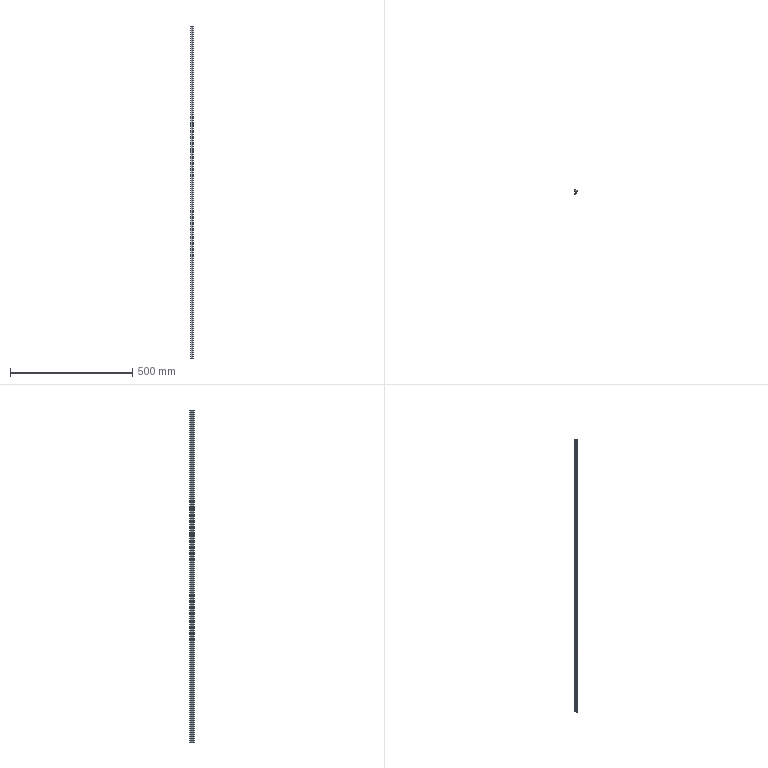Part | SolidWorks | features BaseBody 1, MoveFace 1 | 1 solid | 20 faces | box 10.8 x 17.5 x 1358 mm | volume 107011 mm3 | cylinder 11 | plane 9 | commonest cylinder face diameters 1.6 x2 14 x2 0.4 x1 0.6 x1 0.8 x1 2.6 x1
STEP:
#1=CARTESIAN_POINT('',(-3.236,-11.055,1258.));
#2=VERTEX_POINT('',#1);
#3=CARTESIAN_POINT('',(-4.3,-10.3,1258.));
#4=VERTEX_POINT('',#3);
#5=CARTESIAN_POINT('',(-3.5,-10.3,1258.));
#6=DIRECTION('',(0.,0.,-1.));
#7=DIRECTION('',(1.,0.,0.));
#8=AXIS2_PLACEMENT_3D('',#5,#6,#7);
#9=CIRCLE('',#8,0.8);
#10=EDGE_CURVE('',#2,#4,#9,.T.);
#11=ORIENTED_EDGE('',*,*,#10,.T.);
#12=CARTESIAN_POINT('',(-4.3,-10.3,-100.));
#13=VERTEX_POINT('',#12);
#14=CARTESIAN_POINT('',(-4.3,-10.3,-100.));
#15=DIRECTION('',(0.,0.,-1.));
#16=VECTOR('',#15,1000.);
#17=LINE('',#14,#16);
#18=EDGE_CURVE('',#4,#13,#17,.T.);
#19=ORIENTED_EDGE('',*,*,#18,.T.);
#20=CARTESIAN_POINT('',(-3.236,-11.055,-100.));
#21=VERTEX_POINT('',#20);
#22=CARTESIAN_POINT('',(-3.5,-10.3,-100.));
#23=DIRECTION('',(0.,0.,1.));
#24=DIRECTION('',(-1.,0.,0.));
#25=AXIS2_PLACEMENT_3D('',#22,#23,#24);
#26=CIRCLE('',#25,0.8);
#27=EDGE_CURVE('',#13,#21,#26,.T.);
#28=ORIENTED_EDGE('',*,*,#27,.T.);
#29=CARTESIAN_POINT('',(-3.236,-11.055,-100.));
#30=DIRECTION('',(0.,0.,-1.));
#31=VECTOR('',#30,1000.);
#32=LINE('',#29,#31);
#33=EDGE_CURVE('',#2,#21,#32,.T.);
#34=ORIENTED_EDGE('',*,*,#33,.F.);
#35=EDGE_LOOP('',(#11,#19,#28,#34));
#36=FACE_OUTER_BOUND('',#35,.T.);
#37=CARTESIAN_POINT('',(-3.5,-10.3,-100.));
#38=DIRECTION('',(0.,0.,-1.));
#39=DIRECTION('',(-1.,0.,0.));
#40=AXIS2_PLACEMENT_3D('',#37,#38,#39);
#41=CYLINDRICAL_SURFACE('',#40,0.8);
#42=ADVANCED_FACE('',(#36),#41,.T.);
#43=CARTESIAN_POINT('',(1.184,-6.397,-100.));
#44=VERTEX_POINT('',#43);
#45=CARTESIAN_POINT('',(-5.702,-4.29,-100.));
#46=DIRECTION('',(0.,0.,1.));
#47=DIRECTION('',(-1.,0.,0.));
#48=AXIS2_PLACEMENT_3D('',#45,#46,#47);
#49=CIRCLE('',#48,7.201);
#50=EDGE_CURVE('',#21,#44,#49,.T.);
#51=ORIENTED_EDGE('',*,*,#50,.T.);
#52=CARTESIAN_POINT('',(1.184,-6.397,1258.));
#53=VERTEX_POINT('',#52);
#54=CARTESIAN_POINT('',(1.184,-6.397,-100.));
#55=DIRECTION('',(0.,0.,1.));
#56=VECTOR('',#55,1000.);
#57=LINE('',#54,#56);
#58=EDGE_CURVE('',#44,#53,#57,.T.);
#59=ORIENTED_EDGE('',*,*,#58,.T.);
#60=CARTESIAN_POINT('',(-5.702,-4.29,1258.));
#61=DIRECTION('',(0.,0.,-1.));
#62=DIRECTION('',(1.,0.,0.));
#63=AXIS2_PLACEMENT_3D('',#60,#61,#62);
#64=CIRCLE('',#63,7.201);
#65=EDGE_CURVE('',#53,#2,#64,.T.);
#66=ORIENTED_EDGE('',*,*,#65,.T.);
#67=ORIENTED_EDGE('',*,*,#33,.T.);
#68=EDGE_LOOP('',(#51,#59,#66,#67));
#69=FACE_OUTER_BOUND('',#68,.T.);
#70=CARTESIAN_POINT('',(-5.702,-4.29,-100.));
#71=DIRECTION('',(0.,0.,-1.));
#72=DIRECTION('',(-1.,0.,0.));
#73=AXIS2_PLACEMENT_3D('',#70,#71,#72);
#74=CYLINDRICAL_SURFACE('',#73,7.201);
#75=ADVANCED_FACE('',(#69),#74,.T.);
#76=CARTESIAN_POINT('',(0.9,-6.,-100.));
#77=VERTEX_POINT('',#76);
#78=CARTESIAN_POINT('',(0.9,-6.3,-100.));
#79=DIRECTION('',(0.,0.,1.));
#80=DIRECTION('',(-1.,0.,0.));
#81=AXIS2_PLACEMENT_3D('',#78,#79,#80);
#82=CIRCLE('',#81,0.3);
#83=EDGE_CURVE('',#44,#77,#82,.T.);
#84=ORIENTED_EDGE('',*,*,#83,.T.);
#85=CARTESIAN_POINT('',(0.9,-6.,1258.));
#86=VERTEX_POINT('',#85);
#87=CARTESIAN_POINT('',(0.9,-6.,-100.));
#88=DIRECTION('',(0.,0.,1.));
#89=VECTOR('',#88,1000.);
#90=LINE('',#87,#89);
#91=EDGE_CURVE('',#77,#86,#90,.T.);
#92=ORIENTED_EDGE('',*,*,#91,.T.);
#93=CARTESIAN_POINT('',(0.9,-6.3,1258.));
#94=DIRECTION('',(0.,0.,-1.));
#95=DIRECTION('',(1.,0.,0.));
#96=AXIS2_PLACEMENT_3D('',#93,#94,#95);
#97=CIRCLE('',#96,0.3);
#98=EDGE_CURVE('',#86,#53,#97,.T.);
#99=ORIENTED_EDGE('',*,*,#98,.T.);
#100=ORIENTED_EDGE('',*,*,#58,.F.);
#101=EDGE_LOOP('',(#84,#92,#99,#100));
#102=FACE_OUTER_BOUND('',#101,.T.);
#103=CARTESIAN_POINT('',(0.9,-6.3,-100.));
#104=DIRECTION('',(0.,0.,-1.));
#105=DIRECTION('',(-1.,0.,0.));
#106=AXIS2_PLACEMENT_3D('',#103,#104,#105);
#107=CYLINDRICAL_SURFACE('',#106,0.3);
#108=ADVANCED_FACE('',(#102),#107,.T.);
#109=CARTESIAN_POINT('',(-2.5,-0.5,-100.));
#110=VERTEX_POINT('',#109);
#111=CARTESIAN_POINT('',(-2.5,-6.153,-100.));
#112=VERTEX_POINT('',#111);
#113=CARTESIAN_POINT('',(-2.5,-6.397,-100.));
#114=DIRECTION('',(0.,-1.,0.));
#115=VECTOR('',#114,1000.);
#116=LINE('',#113,#115);
#117=EDGE_CURVE('',#110,#112,#116,.T.);
#118=ORIENTED_EDGE('',*,*,#117,.F.);
#119=CARTESIAN_POINT('',(-4.2,1.695,-100.));
#120=VERTEX_POINT('',#119);
#121=CARTESIAN_POINT('',(-1.701,1.875,-100.));
#122=DIRECTION('',(0.,0.,1.));
#123=DIRECTION('',(-1.,0.,0.));
#124=AXIS2_PLACEMENT_3D('',#121,#122,#123);
#125=CIRCLE('',#124,2.506);
#126=EDGE_CURVE('',#120,#110,#125,.T.);
#127=ORIENTED_EDGE('',*,*,#126,.F.);
#128=CARTESIAN_POINT('',(-4.2,5.1,-100.));
#129=VERTEX_POINT('',#128);
#130=CARTESIAN_POINT('',(-4.2,-6.397,-100.));
#131=DIRECTION('',(0.,-1.,0.));
#132=VECTOR('',#131,1000.);
#133=LINE('',#130,#132);
#134=EDGE_CURVE('',#129,#120,#133,.T.);
#135=ORIENTED_EDGE('',*,*,#134,.F.);
#136=CARTESIAN_POINT('',(-2.892,6.4,-100.));
#137=VERTEX_POINT('',#136);
#138=CARTESIAN_POINT('',(-2.9,5.1,-100.));
#139=DIRECTION('',(0.,0.,1.));
#140=DIRECTION('',(-1.,0.,0.));
#141=AXIS2_PLACEMENT_3D('',#138,#139,#140);
#142=CIRCLE('',#141,1.3);
#143=EDGE_CURVE('',#137,#129,#142,.T.);
#144=ORIENTED_EDGE('',*,*,#143,.F.);
#145=CARTESIAN_POINT('',(0.5,5.5,-100.));
#146=VERTEX_POINT('',#145);
#147=CARTESIAN_POINT('',(-2.934,-0.5999,-100.));
#148=DIRECTION('',(0.,0.,1.));
#149=DIRECTION('',(-1.,0.,0.));
#150=AXIS2_PLACEMENT_3D('',#147,#148,#149);
#151=CIRCLE('',#150,7.);
#152=EDGE_CURVE('',#146,#137,#151,.T.);
#153=ORIENTED_EDGE('',*,*,#152,.F.);
#154=CARTESIAN_POINT('',(5.5,1.7,-100.));
#155=VERTEX_POINT('',#154);
#156=CARTESIAN_POINT('',(5.5,1.7,-100.));
#157=DIRECTION('',(-0.7962,0.6051,0.));
#158=VECTOR('',#157,1000.);
#159=LINE('',#156,#158);
#160=EDGE_CURVE('',#155,#146,#159,.T.);
#161=ORIENTED_EDGE('',*,*,#160,.F.);
#162=CARTESIAN_POINT('',(6.458,-0.2215,-100.));
#163=VERTEX_POINT('',#162);
#164=CARTESIAN_POINT('',(6.458,-0.2215,-100.));
#165=DIRECTION('',(-0.4462,0.8949,0.));
#166=VECTOR('',#165,1000.);
#167=LINE('',#164,#166);
#168=EDGE_CURVE('',#163,#155,#167,.T.);
#169=ORIENTED_EDGE('',*,*,#168,.F.);
#170=CARTESIAN_POINT('',(5.895,-0.7433,-100.));
#171=VERTEX_POINT('',#170);
#172=CARTESIAN_POINT('',(6.1,-0.4,-100.));
#173=DIRECTION('',(0.,0.,1.));
#174=DIRECTION('',(-1.,0.,0.));
#175=AXIS2_PLACEMENT_3D('',#172,#173,#174);
#176=CIRCLE('',#175,0.4);
#177=EDGE_CURVE('',#171,#163,#176,.T.);
#178=ORIENTED_EDGE('',*,*,#177,.F.);
#179=CARTESIAN_POINT('',(3.,0.,-100.));
#180=VERTEX_POINT('',#179);
#181=CARTESIAN_POINT('',(2.746,-6.995,-100.));
#182=DIRECTION('',(0.,0.,-1.));
#183=DIRECTION('',(-1.,0.,0.));
#184=AXIS2_PLACEMENT_3D('',#181,#182,#183);
#185=CIRCLE('',#184,7.);
#186=EDGE_CURVE('',#180,#171,#185,.T.);
#187=ORIENTED_EDGE('',*,*,#186,.F.);
#188=CARTESIAN_POINT('',(0.,0.,-100.));
#189=VERTEX_POINT('',#188);
#190=CARTESIAN_POINT('',(-6.814,0.,-100.));
#191=DIRECTION('',(1.,0.,0.));
#192=VECTOR('',#191,1000.);
#193=LINE('',#190,#192);
#194=EDGE_CURVE('',#189,#180,#193,.T.);
#195=ORIENTED_EDGE('',*,*,#194,.F.);
#196=CARTESIAN_POINT('',(0.,-5.8,-100.));
#197=VERTEX_POINT('',#196);
#198=CARTESIAN_POINT('',(0.,-6.397,-100.));
#199=DIRECTION('',(0.,1.,0.));
#200=VECTOR('',#199,1000.);
#201=LINE('',#198,#200);
#202=EDGE_CURVE('',#197,#189,#201,.T.);
#203=ORIENTED_EDGE('',*,*,#202,.F.);
#204=CARTESIAN_POINT('',(0.2,-6.,-100.));
#205=VERTEX_POINT('',#204);
#206=CARTESIAN_POINT('',(0.2,-5.8,-100.));
#207=DIRECTION('',(0.,0.,1.));
#208=DIRECTION('',(-1.,0.,0.));
#209=AXIS2_PLACEMENT_3D('',#206,#207,#208);
#210=CIRCLE('',#209,0.2);
#211=EDGE_CURVE('',#197,#205,#210,.T.);
#212=ORIENTED_EDGE('',*,*,#211,.T.);
#213=CARTESIAN_POINT('',(-6.814,-6.,-100.));
#214=DIRECTION('',(-1.,0.,0.));
#215=VECTOR('',#214,1000.);
#216=LINE('',#213,#215);
#217=EDGE_CURVE('',#77,#205,#216,.T.);
#218=ORIENTED_EDGE('',*,*,#217,.F.);
#219=ORIENTED_EDGE('',*,*,#83,.F.);
#220=ORIENTED_EDGE('',*,*,#50,.F.);
#221=ORIENTED_EDGE('',*,*,#27,.F.);
#222=CARTESIAN_POINT('',(-3.998,-9.674,-100.));
#223=VERTEX_POINT('',#222);
#224=CARTESIAN_POINT('',(-3.5,-10.3,-100.));
#225=DIRECTION('',(0.,0.,1.));
#226=DIRECTION('',(-1.,0.,0.));
#227=AXIS2_PLACEMENT_3D('',#224,#225,#226);
#228=CIRCLE('',#227,0.8);
#229=EDGE_CURVE('',#223,#13,#228,.T.);
#230=ORIENTED_EDGE('',*,*,#229,.F.);
#231=CARTESIAN_POINT('',(-6.814,-6.397,-100.));
#232=DIRECTION('',(0.,0.,-1.));
#233=DIRECTION('',(-1.,0.,0.));
#234=AXIS2_PLACEMENT_3D('',#231,#232,#233);
#235=CIRCLE('',#234,4.321);
#236=EDGE_CURVE('',#112,#223,#235,.T.);
#237=ORIENTED_EDGE('',*,*,#236,.F.);
#238=EDGE_LOOP('',(#118,#127,#135,#144,#153,#161,#169,#178,#187,#195,#203,#212,#218,#219,#220,#221,#230,#237));
#239=FACE_OUTER_BOUND('',#238,.T.);
#240=CARTESIAN_POINT('',(-6.814,-6.397,-100.));
#241=DIRECTION('',(0.,0.,1.));
#242=DIRECTION('',(1.,0.,0.));
#243=AXIS2_PLACEMENT_3D('',#240,#241,#242);
#244=PLANE('',#243);
#245=ADVANCED_FACE('',(#239),#244,.F.);
#246=ORIENTED_EDGE('',*,*,#18,.F.);
#247=CARTESIAN_POINT('',(-3.998,-9.674,1258.));
#248=VERTEX_POINT('',#247);
#249=CARTESIAN_POINT('',(-3.5,-10.3,1258.));
#250=DIRECTION('',(0.,0.,-1.));
#251=DIRECTION('',(1.,0.,0.));
#252=AXIS2_PLACEMENT_3D('',#249,#250,#251);
#253=CIRCLE('',#252,0.8);
#254=EDGE_CURVE('',#4,#248,#253,.T.);
#255=ORIENTED_EDGE('',*,*,#254,.T.);
#256=CARTESIAN_POINT('',(-3.998,-9.674,-100.));
#257=DIRECTION('',(0.,0.,-1.));
#258=VECTOR('',#257,1000.);
#259=LINE('',#256,#258);
#260=EDGE_CURVE('',#248,#223,#259,.T.);
#261=ORIENTED_EDGE('',*,*,#260,.T.);
#262=ORIENTED_EDGE('',*,*,#229,.T.);
#263=EDGE_LOOP('',(#246,#255,#261,#262));
#264=FACE_OUTER_BOUND('',#263,.T.);
#265=CARTESIAN_POINT('',(-3.5,-10.3,-100.));
#266=DIRECTION('',(0.,0.,-1.));
#267=DIRECTION('',(-1.,0.,0.));
#268=AXIS2_PLACEMENT_3D('',#265,#266,#267);
#269=CYLINDRICAL_SURFACE('',#268,0.8);
#270=ADVANCED_FACE('',(#264),#269,.T.);
#271=CARTESIAN_POINT('',(-4.2,1.695,1258.));
#272=VERTEX_POINT('',#271);
#273=CARTESIAN_POINT('',(-2.5,-0.5,1258.));
#274=VERTEX_POINT('',#273);
#275=CARTESIAN_POINT('',(-1.701,1.875,1258.));
#276=DIRECTION('',(0.,0.,1.));
#277=DIRECTION('',(1.,0.,0.));
#278=AXIS2_PLACEMENT_3D('',#275,#276,#277);
#279=CIRCLE('',#278,2.506);
#280=EDGE_CURVE('',#272,#274,#279,.T.);
#281=ORIENTED_EDGE('',*,*,#280,.T.);
#282=CARTESIAN_POINT('',(-2.5,-6.153,1258.));
#283=VERTEX_POINT('',#282);
#284=CARTESIAN_POINT('',(-2.5,-6.397,1258.));
#285=DIRECTION('',(0.,-1.,0.));
#286=VECTOR('',#285,1000.);
#287=LINE('',#284,#286);
#288=EDGE_CURVE('',#274,#283,#287,.T.);
#289=ORIENTED_EDGE('',*,*,#288,.T.);
#290=CARTESIAN_POINT('',(-6.814,-6.397,1258.));
#291=DIRECTION('',(0.,0.,-1.));
#292=DIRECTION('',(1.,0.,0.));
#293=AXIS2_PLACEMENT_3D('',#290,#291,#292);
#294=CIRCLE('',#293,4.321);
#295=EDGE_CURVE('',#283,#248,#294,.T.);
#296=ORIENTED_EDGE('',*,*,#295,.T.);
#297=ORIENTED_EDGE('',*,*,#254,.F.);
#298=ORIENTED_EDGE('',*,*,#10,.F.);
#299=ORIENTED_EDGE('',*,*,#65,.F.);
#300=ORIENTED_EDGE('',*,*,#98,.F.);
#301=CARTESIAN_POINT('',(0.2,-6.,1258.));
#302=VERTEX_POINT('',#301);
#303=CARTESIAN_POINT('',(-6.814,-6.,1258.));
#304=DIRECTION('',(-1.,0.,0.));
#305=VECTOR('',#304,1000.);
#306=LINE('',#303,#305);
#307=EDGE_CURVE('',#86,#302,#306,.T.);
#308=ORIENTED_EDGE('',*,*,#307,.T.);
#309=CARTESIAN_POINT('',(0.,-5.8,1258.));
#310=VERTEX_POINT('',#309);
#311=CARTESIAN_POINT('',(0.2,-5.8,1258.));
#312=DIRECTION('',(0.,0.,-1.));
#313=DIRECTION('',(1.,0.,0.));
#314=AXIS2_PLACEMENT_3D('',#311,#312,#313);
#315=CIRCLE('',#314,0.2);
#316=EDGE_CURVE('',#302,#310,#315,.T.);
#317=ORIENTED_EDGE('',*,*,#316,.T.);
#318=CARTESIAN_POINT('',(0.,0.,1258.));
#319=VERTEX_POINT('',#318);
#320=CARTESIAN_POINT('',(0.,-6.397,1258.));
#321=DIRECTION('',(0.,1.,0.));
#322=VECTOR('',#321,1000.);
#323=LINE('',#320,#322);
#324=EDGE_CURVE('',#310,#319,#323,.T.);
#325=ORIENTED_EDGE('',*,*,#324,.T.);
#326=CARTESIAN_POINT('',(3.,0.,1258.));
#327=VERTEX_POINT('',#326);
#328=CARTESIAN_POINT('',(-6.814,0.,1258.));
#329=DIRECTION('',(1.,0.,0.));
#330=VECTOR('',#329,1000.);
#331=LINE('',#328,#330);
#332=EDGE_CURVE('',#319,#327,#331,.T.);
#333=ORIENTED_EDGE('',*,*,#332,.T.);
#334=CARTESIAN_POINT('',(5.895,-0.7433,1258.));
#335=VERTEX_POINT('',#334);
#336=CARTESIAN_POINT('',(2.746,-6.995,1258.));
#337=DIRECTION('',(0.,0.,-1.));
#338=DIRECTION('',(1.,0.,0.));
#339=AXIS2_PLACEMENT_3D('',#336,#337,#338);
#340=CIRCLE('',#339,7.);
#341=EDGE_CURVE('',#327,#335,#340,.T.);
#342=ORIENTED_EDGE('',*,*,#341,.T.);
#343=CARTESIAN_POINT('',(6.458,-0.2215,1258.));
#344=VERTEX_POINT('',#343);
#345=CARTESIAN_POINT('',(6.1,-0.4,1258.));
#346=DIRECTION('',(0.,0.,-1.));
#347=DIRECTION('',(1.,0.,0.));
#348=AXIS2_PLACEMENT_3D('',#345,#346,#347);
#349=CIRCLE('',#348,0.4);
#350=EDGE_CURVE('',#344,#335,#349,.T.);
#351=ORIENTED_EDGE('',*,*,#350,.F.);
#352=CARTESIAN_POINT('',(5.5,1.7,1258.));
#353=VERTEX_POINT('',#352);
#354=CARTESIAN_POINT('',(6.282,0.1323,1258.));
#355=DIRECTION('',(-0.4462,0.8949,0.));
#356=VECTOR('',#355,1000.);
#357=LINE('',#354,#356);
#358=EDGE_CURVE('',#344,#353,#357,.T.);
#359=ORIENTED_EDGE('',*,*,#358,.T.);
#360=CARTESIAN_POINT('',(0.5,5.5,1258.));
#361=VERTEX_POINT('',#360);
#362=CARTESIAN_POINT('',(1.595,4.668,1258.));
#363=DIRECTION('',(-0.7962,0.6051,0.));
#364=VECTOR('',#363,1000.);
#365=LINE('',#362,#364);
#366=EDGE_CURVE('',#353,#361,#365,.T.);
#367=ORIENTED_EDGE('',*,*,#366,.T.);
#368=CARTESIAN_POINT('',(-2.892,6.4,1258.));
#369=VERTEX_POINT('',#368);
#370=CARTESIAN_POINT('',(-2.934,-0.5999,1258.));
#371=DIRECTION('',(0.,0.,1.));
#372=DIRECTION('',(1.,0.,0.));
#373=AXIS2_PLACEMENT_3D('',#370,#371,#372);
#374=CIRCLE('',#373,7.);
#375=EDGE_CURVE('',#361,#369,#374,.T.);
#376=ORIENTED_EDGE('',*,*,#375,.T.);
#377=CARTESIAN_POINT('',(-4.2,5.1,1258.));
#378=VERTEX_POINT('',#377);
#379=CARTESIAN_POINT('',(-2.9,5.1,1258.));
#380=DIRECTION('',(0.,0.,1.));
#381=DIRECTION('',(1.,0.,0.));
#382=AXIS2_PLACEMENT_3D('',#379,#380,#381);
#383=CIRCLE('',#382,1.3);
#384=EDGE_CURVE('',#369,#378,#383,.T.);
#385=ORIENTED_EDGE('',*,*,#384,.T.);
#386=CARTESIAN_POINT('',(-4.2,-6.397,1258.));
#387=DIRECTION('',(0.,-1.,0.));
#388=VECTOR('',#387,1000.);
#389=LINE('',#386,#388);
#390=EDGE_CURVE('',#378,#272,#389,.T.);
#391=ORIENTED_EDGE('',*,*,#390,.T.);
#392=EDGE_LOOP('',(#281,#289,#296,#297,#298,#299,#300,#308,#317,#325,#333,#342,#351,#359,#367,#376,#385,#391));
#393=FACE_OUTER_BOUND('',#392,.T.);
#394=CARTESIAN_POINT('',(-6.814,-6.397,1258.));
#395=DIRECTION('',(0.,0.,1.));
#396=DIRECTION('',(1.,0.,0.));
#397=AXIS2_PLACEMENT_3D('',#394,#395,#396);
#398=PLANE('',#397);
#399=ADVANCED_FACE('',(#393),#398,.T.);
#400=ORIENTED_EDGE('',*,*,#217,.T.);
#401=CARTESIAN_POINT('',(0.2,-6.,-100.));
#402=DIRECTION('',(0.,0.,1.));
#403=VECTOR('',#402,1000.);
#404=LINE('',#401,#403);
#405=EDGE_CURVE('',#205,#302,#404,.T.);
#406=ORIENTED_EDGE('',*,*,#405,.T.);
#407=ORIENTED_EDGE('',*,*,#307,.F.);
#408=ORIENTED_EDGE('',*,*,#91,.F.);
#409=EDGE_LOOP('',(#400,#406,#407,#408));
#410=FACE_OUTER_BOUND('',#409,.T.);
#411=CARTESIAN_POINT('',(0.9,-6.,-100.));
#412=DIRECTION('',(0.,1.,0.));
#413=DIRECTION('',(0.,0.,1.));
#414=AXIS2_PLACEMENT_3D('',#411,#412,#413);
#415=PLANE('',#414);
#416=ADVANCED_FACE('',(#410),#415,.T.);
#417=CARTESIAN_POINT('',(-2.5,-6.153,-100.));
#418=DIRECTION('',(0.,0.,1.));
#419=VECTOR('',#418,1000.);
#420=LINE('',#417,#419);
#421=EDGE_CURVE('',#112,#283,#420,.T.);
#422=ORIENTED_EDGE('',*,*,#421,.F.);
#423=ORIENTED_EDGE('',*,*,#236,.T.);
#424=ORIENTED_EDGE('',*,*,#260,.F.);
#425=ORIENTED_EDGE('',*,*,#295,.F.);
#426=EDGE_LOOP('',(#422,#423,#424,#425));
#427=FACE_OUTER_BOUND('',#426,.T.);
#428=CARTESIAN_POINT('',(-6.814,-6.397,-100.));
#429=DIRECTION('',(0.,0.,-1.));
#430=DIRECTION('',(-1.,0.,0.));
#431=AXIS2_PLACEMENT_3D('',#428,#429,#430);
#432=CYLINDRICAL_SURFACE('',#431,4.321);
#433=ADVANCED_FACE('',(#427),#432,.F.);
#434=ORIENTED_EDGE('',*,*,#117,.T.);
#435=ORIENTED_EDGE('',*,*,#421,.T.);
#436=ORIENTED_EDGE('',*,*,#288,.F.);
#437=CARTESIAN_POINT('',(-2.5,-0.5,-100.));
#438=DIRECTION('',(0.,0.,-1.));
#439=VECTOR('',#438,1000.);
#440=LINE('',#437,#439);
#441=EDGE_CURVE('',#274,#110,#440,.T.);
#442=ORIENTED_EDGE('',*,*,#441,.T.);
#443=EDGE_LOOP('',(#434,#435,#436,#442));
#444=FACE_OUTER_BOUND('',#443,.T.);
#445=CARTESIAN_POINT('',(-2.5,-0.5,-100.));
#446=DIRECTION('',(-1.,0.,0.));
#447=DIRECTION('',(0.,0.,1.));
#448=AXIS2_PLACEMENT_3D('',#445,#446,#447);
#449=PLANE('',#448);
#450=ADVANCED_FACE('',(#444),#449,.T.);
#451=ORIENTED_EDGE('',*,*,#126,.T.);
#452=ORIENTED_EDGE('',*,*,#441,.F.);
#453=ORIENTED_EDGE('',*,*,#280,.F.);
#454=CARTESIAN_POINT('',(-4.2,1.695,-100.));
#455=DIRECTION('',(0.,0.,-1.));
#456=VECTOR('',#455,1000.);
#457=LINE('',#454,#456);
#458=EDGE_CURVE('',#272,#120,#457,.T.);
#459=ORIENTED_EDGE('',*,*,#458,.T.);
#460=EDGE_LOOP('',(#451,#452,#453,#459));
#461=FACE_OUTER_BOUND('',#460,.T.);
#462=CARTESIAN_POINT('',(-1.701,1.875,-100.));
#463=DIRECTION('',(0.,0.,-1.));
#464=DIRECTION('',(-1.,0.,0.));
#465=AXIS2_PLACEMENT_3D('',#462,#463,#464);
#466=CYLINDRICAL_SURFACE('',#465,2.506);
#467=ADVANCED_FACE('',(#461),#466,.T.);
#468=ORIENTED_EDGE('',*,*,#134,.T.);
#469=ORIENTED_EDGE('',*,*,#458,.F.);
#470=ORIENTED_EDGE('',*,*,#390,.F.);
#471=CARTESIAN_POINT('',(-4.2,5.1,-100.));
#472=DIRECTION('',(0.,0.,-1.));
#473=VECTOR('',#472,1000.);
#474=LINE('',#471,#473);
#475=EDGE_CURVE('',#378,#129,#474,.T.);
#476=ORIENTED_EDGE('',*,*,#475,.T.);
#477=EDGE_LOOP('',(#468,#469,#470,#476));
#478=FACE_OUTER_BOUND('',#477,.T.);
#479=CARTESIAN_POINT('',(-4.2,5.1,-100.));
#480=DIRECTION('',(-1.,0.,0.));
#481=DIRECTION('',(0.,0.,1.));
#482=AXIS2_PLACEMENT_3D('',#479,#480,#481);
#483=PLANE('',#482);
#484=ADVANCED_FACE('',(#478),#483,.T.);
#485=ORIENTED_EDGE('',*,*,#143,.T.);
#486=ORIENTED_EDGE('',*,*,#475,.F.);
#487=ORIENTED_EDGE('',*,*,#384,.F.);
#488=CARTESIAN_POINT('',(-2.892,6.4,-100.));
#489=DIRECTION('',(0.,0.,-1.));
#490=VECTOR('',#489,1000.);
#491=LINE('',#488,#490);
#492=EDGE_CURVE('',#369,#137,#491,.T.);
#493=ORIENTED_EDGE('',*,*,#492,.T.);
#494=EDGE_LOOP('',(#485,#486,#487,#493));
#495=FACE_OUTER_BOUND('',#494,.T.);
#496=CARTESIAN_POINT('',(-2.9,5.1,-100.));
#497=DIRECTION('',(0.,0.,-1.));
#498=DIRECTION('',(-1.,0.,0.));
#499=AXIS2_PLACEMENT_3D('',#496,#497,#498);
#500=CYLINDRICAL_SURFACE('',#499,1.3);
#501=ADVANCED_FACE('',(#495),#500,.T.);
#502=ORIENTED_EDGE('',*,*,#152,.T.);
#503=ORIENTED_EDGE('',*,*,#492,.F.);
#504=ORIENTED_EDGE('',*,*,#375,.F.);
#505=CARTESIAN_POINT('',(0.5,5.5,-100.));
#506=DIRECTION('',(0.,0.,-1.));
#507=VECTOR('',#506,1000.);
#508=LINE('',#505,#507);
#509=EDGE_CURVE('',#361,#146,#508,.T.);
#510=ORIENTED_EDGE('',*,*,#509,.T.);
#511=EDGE_LOOP('',(#502,#503,#504,#510));
#512=FACE_OUTER_BOUND('',#511,.T.);
#513=CARTESIAN_POINT('',(-2.934,-0.5999,-100.));
#514=DIRECTION('',(0.,0.,-1.));
#515=DIRECTION('',(-1.,0.,0.));
#516=AXIS2_PLACEMENT_3D('',#513,#514,#515);
#517=CYLINDRICAL_SURFACE('',#516,7.);
#518=ADVANCED_FACE('',(#512),#517,.T.);
#519=ORIENTED_EDGE('',*,*,#160,.T.);
#520=ORIENTED_EDGE('',*,*,#509,.F.);
#521=ORIENTED_EDGE('',*,*,#366,.F.);
#522=CARTESIAN_POINT('',(5.5,1.7,-100.));
#523=DIRECTION('',(0.,0.,-1.));
#524=VECTOR('',#523,1000.);
#525=LINE('',#522,#524);
#526=EDGE_CURVE('',#353,#155,#525,.T.);
#527=ORIENTED_EDGE('',*,*,#526,.T.);
#528=EDGE_LOOP('',(#519,#520,#521,#527));
#529=FACE_OUTER_BOUND('',#528,.T.);
#530=CARTESIAN_POINT('',(5.5,1.7,-100.));
#531=DIRECTION('',(0.6051,0.7962,0.));
#532=DIRECTION('',(-0.7962,0.6051,0.));
#533=AXIS2_PLACEMENT_3D('',#530,#531,#532);
#534=PLANE('',#533);
#535=ADVANCED_FACE('',(#529),#534,.T.);
#536=ORIENTED_EDGE('',*,*,#168,.T.);
#537=ORIENTED_EDGE('',*,*,#526,.F.);
#538=ORIENTED_EDGE('',*,*,#358,.F.);
#539=CARTESIAN_POINT('',(6.458,-0.2215,-100.));
#540=DIRECTION('',(0.,0.,-1.));
#541=VECTOR('',#540,1000.);
#542=LINE('',#539,#541);
#543=EDGE_CURVE('',#344,#163,#542,.T.);
#544=ORIENTED_EDGE('',*,*,#543,.T.);
#545=EDGE_LOOP('',(#536,#537,#538,#544));
#546=FACE_OUTER_BOUND('',#545,.T.);
#547=CARTESIAN_POINT('',(6.458,-0.2215,-100.));
#548=DIRECTION('',(0.8949,0.4462,0.));
#549=DIRECTION('',(-0.4462,0.8949,0.));
#550=AXIS2_PLACEMENT_3D('',#547,#548,#549);
#551=PLANE('',#550);
#552=ADVANCED_FACE('',(#546),#551,.T.);
#553=CARTESIAN_POINT('',(3.,0.,-100.));
#554=DIRECTION('',(0.,0.,1.));
#555=VECTOR('',#554,1000.);
#556=LINE('',#553,#555);
#557=EDGE_CURVE('',#180,#327,#556,.T.);
#558=ORIENTED_EDGE('',*,*,#557,.F.);
#559=ORIENTED_EDGE('',*,*,#186,.T.);
#560=CARTESIAN_POINT('',(5.895,-0.7433,-100.));
#561=DIRECTION('',(0.,0.,-1.));
#562=VECTOR('',#561,1000.);
#563=LINE('',#560,#562);
#564=EDGE_CURVE('',#335,#171,#563,.T.);
#565=ORIENTED_EDGE('',*,*,#564,.F.);
#566=ORIENTED_EDGE('',*,*,#341,.F.);
#567=EDGE_LOOP('',(#558,#559,#565,#566));
#568=FACE_OUTER_BOUND('',#567,.T.);
#569=CARTESIAN_POINT('',(2.746,-6.995,-100.));
#570=DIRECTION('',(0.,0.,-1.));
#571=DIRECTION('',(-1.,0.,0.));
#572=AXIS2_PLACEMENT_3D('',#569,#570,#571);
#573=CYLINDRICAL_SURFACE('',#572,7.);
#574=ADVANCED_FACE('',(#568),#573,.F.);
#575=ORIENTED_EDGE('',*,*,#194,.T.);
#576=ORIENTED_EDGE('',*,*,#557,.T.);
#577=ORIENTED_EDGE('',*,*,#332,.F.);
#578=CARTESIAN_POINT('',(0.,0.,-100.));
#579=DIRECTION('',(0.,0.,-1.));
#580=VECTOR('',#579,1000.);
#581=LINE('',#578,#580);
#582=EDGE_CURVE('',#319,#189,#581,.T.);
#583=ORIENTED_EDGE('',*,*,#582,.T.);
#584=EDGE_LOOP('',(#575,#576,#577,#583));
#585=FACE_OUTER_BOUND('',#584,.T.);
#586=CARTESIAN_POINT('',(0.,0.,-100.));
#587=DIRECTION('',(0.,-1.,0.));
#588=DIRECTION('',(0.,0.,-1.));
#589=AXIS2_PLACEMENT_3D('',#586,#587,#588);
#590=PLANE('',#589);
#591=ADVANCED_FACE('',(#585),#590,.T.);
#592=ORIENTED_EDGE('',*,*,#202,.T.);
#593=ORIENTED_EDGE('',*,*,#582,.F.);
#594=ORIENTED_EDGE('',*,*,#324,.F.);
#595=CARTESIAN_POINT('',(0.,-5.8,-100.));
#596=DIRECTION('',(0.,0.,-1.));
#597=VECTOR('',#596,1000.);
#598=LINE('',#595,#597);
#599=EDGE_CURVE('',#310,#197,#598,.T.);
#600=ORIENTED_EDGE('',*,*,#599,.T.);
#601=EDGE_LOOP('',(#592,#593,#594,#600));
#602=FACE_OUTER_BOUND('',#601,.T.);
#603=CARTESIAN_POINT('',(0.,-5.8,-100.));
#604=DIRECTION('',(1.,0.,0.));
#605=DIRECTION('',(0.,0.,-1.));
#606=AXIS2_PLACEMENT_3D('',#603,#604,#605);
#607=PLANE('',#606);
#608=ADVANCED_FACE('',(#602),#607,.T.);
#609=ORIENTED_EDGE('',*,*,#405,.F.);
#610=ORIENTED_EDGE('',*,*,#211,.F.);
#611=ORIENTED_EDGE('',*,*,#599,.F.);
#612=ORIENTED_EDGE('',*,*,#316,.F.);
#613=EDGE_LOOP('',(#609,#610,#611,#612));
#614=FACE_OUTER_BOUND('',#613,.T.);
#615=CARTESIAN_POINT('',(0.2,-5.8,-100.));
#616=DIRECTION('',(0.,0.,-1.));
#617=DIRECTION('',(-1.,0.,0.));
#618=AXIS2_PLACEMENT_3D('',#615,#616,#617);
#619=CYLINDRICAL_SURFACE('',#618,0.2);
#620=ADVANCED_FACE('',(#614),#619,.F.);
#621=ORIENTED_EDGE('',*,*,#177,.T.);
#622=ORIENTED_EDGE('',*,*,#543,.F.);
#623=ORIENTED_EDGE('',*,*,#350,.T.);
#624=ORIENTED_EDGE('',*,*,#564,.T.);
#625=EDGE_LOOP('',(#621,#622,#623,#624));
#626=FACE_OUTER_BOUND('',#625,.T.);
#627=CARTESIAN_POINT('',(6.1,-0.4,-100.));
#628=DIRECTION('',(0.,0.,-1.));
#629=DIRECTION('',(-1.,0.,0.));
#630=AXIS2_PLACEMENT_3D('',#627,#628,#629);
#631=CYLINDRICAL_SURFACE('',#630,0.4);
#632=ADVANCED_FACE('',(#626),#631,.T.);
#633=CLOSED_SHELL('',(#42,#75,#108,#245,#270,#399,#416,#433,#450,#467,#484,#501,#518,#535,#552,#574,#591,#608,#620,#632));
#634=MANIFOLD_SOLID_BREP('',#633);
#635=CARTESIAN_POINT('',(0.,0.,0.));
#636=DIRECTION('',(0.,0.,1.));
#637=DIRECTION('',(1.,0.,0.));
#638=AXIS2_PLACEMENT_3D('',#635,#636,#637);
#639=(LENGTH_UNIT()NAMED_UNIT(*)SI_UNIT(.MILLI.,.METRE.));
#640=UNCERTAINTY_MEASURE_WITH_UNIT(LENGTH_MEASURE(0.00001),#639,'','');
#641=(NAMED_UNIT(*)PLANE_ANGLE_UNIT()SI_UNIT($,.RADIAN.));
#642=(NAMED_UNIT(*)SI_UNIT($,.STERADIAN.)SOLID_ANGLE_UNIT());
#643=(GEOMETRIC_REPRESENTATION_CONTEXT(3)GLOBAL_UNCERTAINTY_ASSIGNED_CONTEXT((#640))GLOBAL_UNIT_ASSIGNED_CONTEXT((#639,#641,#642))REPRESENTATION_CONTEXT('',''));
#644=ADVANCED_BREP_SHAPE_REPRESENTATION('',(#634,#638),#643);